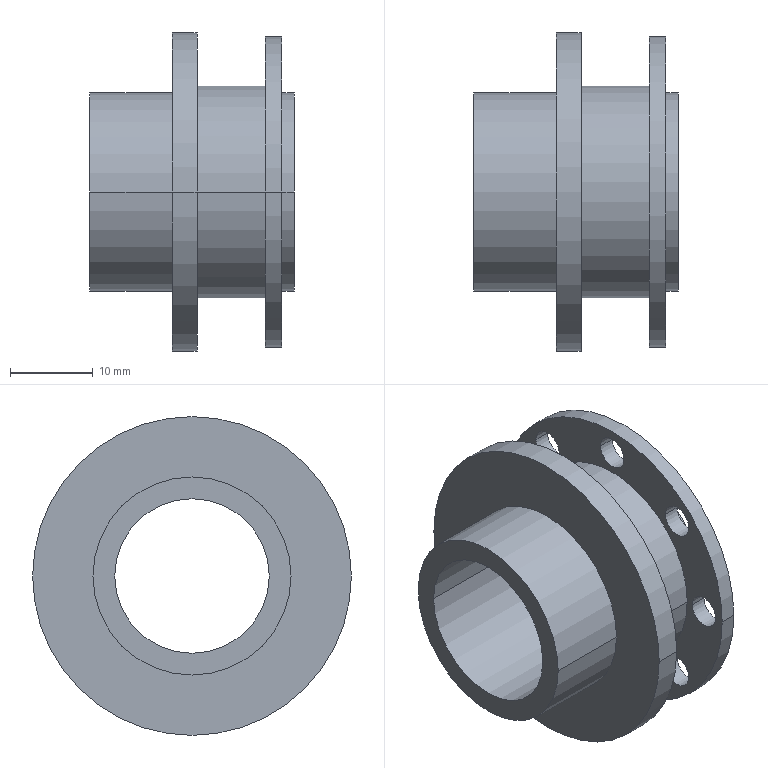Part | SolidWorks | features SavedExtBody 1 | 1 solid | 34 faces | box 24.772 x 38.609 x 38.609 mm | volume 8203 mm3 | cylinder 28 | plane 6 | commonest cylinder face diameters 4 x16 24 x4 18.724 x2 25.677 x2 37.649 x2 38.609 x2
STEP:
#1=CARTESIAN_POINT('',(-65.,13.695,65.));
#2=VERTEX_POINT('',#1);
#3=CARTESIAN_POINT('',(-65.,17.695,65.));
#4=VERTEX_POINT('',#3);
#5=CARTESIAN_POINT('',(-65.,15.695,65.));
#6=DIRECTION('',(1.,0.,0.));
#7=DIRECTION('',(0.,-1.,0.));
#8=AXIS2_PLACEMENT_3D('',#5,#6,#7);
#9=CIRCLE('',#8,2.);
#10=EDGE_CURVE('',#2,#4,#9,.T.);
#11=ORIENTED_EDGE('',*,*,#10,.T.);
#12=CARTESIAN_POINT('',(-67.,17.695,65.));
#13=VERTEX_POINT('',#12);
#14=CARTESIAN_POINT('',(-59.343,17.695,65.));
#15=DIRECTION('',(-1.,0.,0.));
#16=VECTOR('',#15,1000.);
#17=LINE('',#14,#16);
#18=EDGE_CURVE('',#4,#13,#17,.T.);
#19=ORIENTED_EDGE('',*,*,#18,.T.);
#20=CARTESIAN_POINT('',(-67.,13.695,65.));
#21=VERTEX_POINT('',#20);
#22=CARTESIAN_POINT('',(-67.,15.695,65.));
#23=DIRECTION('',(-1.,0.,0.));
#24=DIRECTION('',(0.,-1.,0.));
#25=AXIS2_PLACEMENT_3D('',#22,#23,#24);
#26=CIRCLE('',#25,2.);
#27=EDGE_CURVE('',#13,#21,#26,.T.);
#28=ORIENTED_EDGE('',*,*,#27,.T.);
#29=CARTESIAN_POINT('',(-59.343,13.695,65.));
#30=DIRECTION('',(-1.,0.,0.));
#31=VECTOR('',#30,1000.);
#32=LINE('',#29,#31);
#33=EDGE_CURVE('',#2,#21,#32,.T.);
#34=ORIENTED_EDGE('',*,*,#33,.F.);
#35=EDGE_LOOP('',(#11,#19,#28,#34));
#36=FACE_OUTER_BOUND('',#35,.T.);
#37=CARTESIAN_POINT('',(-59.343,15.695,65.));
#38=DIRECTION('',(-1.,0.,0.));
#39=DIRECTION('',(0.,-1.,0.));
#40=AXIS2_PLACEMENT_3D('',#37,#38,#39);
#41=CYLINDRICAL_SURFACE('',#40,2.);
#42=ADVANCED_FACE('',(#36),#41,.F.);
#43=CARTESIAN_POINT('',(-65.,9.098,76.098));
#44=VERTEX_POINT('',#43);
#45=CARTESIAN_POINT('',(-65.,13.098,76.098));
#46=VERTEX_POINT('',#45);
#47=CARTESIAN_POINT('',(-65.,11.098,76.098));
#48=DIRECTION('',(1.,0.,0.));
#49=DIRECTION('',(0.,-1.,0.));
#50=AXIS2_PLACEMENT_3D('',#47,#48,#49);
#51=CIRCLE('',#50,2.);
#52=EDGE_CURVE('',#44,#46,#51,.T.);
#53=ORIENTED_EDGE('',*,*,#52,.T.);
#54=CARTESIAN_POINT('',(-67.,13.098,76.098));
#55=VERTEX_POINT('',#54);
#56=CARTESIAN_POINT('',(-59.343,13.098,76.098));
#57=DIRECTION('',(-1.,0.,0.));
#58=VECTOR('',#57,1000.);
#59=LINE('',#56,#58);
#60=EDGE_CURVE('',#46,#55,#59,.T.);
#61=ORIENTED_EDGE('',*,*,#60,.T.);
#62=CARTESIAN_POINT('',(-67.,9.098,76.098));
#63=VERTEX_POINT('',#62);
#64=CARTESIAN_POINT('',(-67.,11.098,76.098));
#65=DIRECTION('',(-1.,0.,0.));
#66=DIRECTION('',(0.,-1.,0.));
#67=AXIS2_PLACEMENT_3D('',#64,#65,#66);
#68=CIRCLE('',#67,2.);
#69=EDGE_CURVE('',#55,#63,#68,.T.);
#70=ORIENTED_EDGE('',*,*,#69,.T.);
#71=CARTESIAN_POINT('',(-59.343,9.098,76.098));
#72=DIRECTION('',(-1.,0.,0.));
#73=VECTOR('',#72,1000.);
#74=LINE('',#71,#73);
#75=EDGE_CURVE('',#44,#63,#74,.T.);
#76=ORIENTED_EDGE('',*,*,#75,.F.);
#77=EDGE_LOOP('',(#53,#61,#70,#76));
#78=FACE_OUTER_BOUND('',#77,.T.);
#79=CARTESIAN_POINT('',(-59.343,11.098,76.098));
#80=DIRECTION('',(-1.,0.,0.));
#81=DIRECTION('',(0.,-1.,0.));
#82=AXIS2_PLACEMENT_3D('',#79,#80,#81);
#83=CYLINDRICAL_SURFACE('',#82,2.);
#84=ADVANCED_FACE('',(#78),#83,.F.);
#85=CARTESIAN_POINT('',(-65.,-2.,80.695));
#86=VERTEX_POINT('',#85);
#87=CARTESIAN_POINT('',(-65.,2.,80.695));
#88=VERTEX_POINT('',#87);
#89=CARTESIAN_POINT('',(-65.,0.,80.695));
#90=DIRECTION('',(1.,0.,0.));
#91=DIRECTION('',(0.,-1.,0.));
#92=AXIS2_PLACEMENT_3D('',#89,#90,#91);
#93=CIRCLE('',#92,2.);
#94=EDGE_CURVE('',#86,#88,#93,.T.);
#95=ORIENTED_EDGE('',*,*,#94,.T.);
#96=CARTESIAN_POINT('',(-67.,2.,80.695));
#97=VERTEX_POINT('',#96);
#98=CARTESIAN_POINT('',(-59.343,2.,80.695));
#99=DIRECTION('',(-1.,0.,0.));
#100=VECTOR('',#99,1000.);
#101=LINE('',#98,#100);
#102=EDGE_CURVE('',#88,#97,#101,.T.);
#103=ORIENTED_EDGE('',*,*,#102,.T.);
#104=CARTESIAN_POINT('',(-67.,-2.,80.695));
#105=VERTEX_POINT('',#104);
#106=CARTESIAN_POINT('',(-67.,0.,80.695));
#107=DIRECTION('',(-1.,0.,0.));
#108=DIRECTION('',(0.,-1.,0.));
#109=AXIS2_PLACEMENT_3D('',#106,#107,#108);
#110=CIRCLE('',#109,2.);
#111=EDGE_CURVE('',#97,#105,#110,.T.);
#112=ORIENTED_EDGE('',*,*,#111,.T.);
#113=CARTESIAN_POINT('',(-59.343,-2.,80.695));
#114=DIRECTION('',(-1.,0.,0.));
#115=VECTOR('',#114,1000.);
#116=LINE('',#113,#115);
#117=EDGE_CURVE('',#86,#105,#116,.T.);
#118=ORIENTED_EDGE('',*,*,#117,.F.);
#119=EDGE_LOOP('',(#95,#103,#112,#118));
#120=FACE_OUTER_BOUND('',#119,.T.);
#121=CARTESIAN_POINT('',(-59.343,0.,80.695));
#122=DIRECTION('',(-1.,0.,0.));
#123=DIRECTION('',(0.,-1.,0.));
#124=AXIS2_PLACEMENT_3D('',#121,#122,#123);
#125=CYLINDRICAL_SURFACE('',#124,2.);
#126=ADVANCED_FACE('',(#120),#125,.F.);
#127=CARTESIAN_POINT('',(-65.,-13.098,76.098));
#128=VERTEX_POINT('',#127);
#129=CARTESIAN_POINT('',(-65.,-9.098,76.098));
#130=VERTEX_POINT('',#129);
#131=CARTESIAN_POINT('',(-65.,-11.098,76.098));
#132=DIRECTION('',(1.,0.,0.));
#133=DIRECTION('',(0.,-1.,0.));
#134=AXIS2_PLACEMENT_3D('',#131,#132,#133);
#135=CIRCLE('',#134,2.);
#136=EDGE_CURVE('',#128,#130,#135,.T.);
#137=ORIENTED_EDGE('',*,*,#136,.T.);
#138=CARTESIAN_POINT('',(-67.,-9.098,76.098));
#139=VERTEX_POINT('',#138);
#140=CARTESIAN_POINT('',(-59.343,-9.098,76.098));
#141=DIRECTION('',(-1.,0.,0.));
#142=VECTOR('',#141,1000.);
#143=LINE('',#140,#142);
#144=EDGE_CURVE('',#130,#139,#143,.T.);
#145=ORIENTED_EDGE('',*,*,#144,.T.);
#146=CARTESIAN_POINT('',(-67.,-13.098,76.098));
#147=VERTEX_POINT('',#146);
#148=CARTESIAN_POINT('',(-67.,-11.098,76.098));
#149=DIRECTION('',(-1.,0.,0.));
#150=DIRECTION('',(0.,-1.,0.));
#151=AXIS2_PLACEMENT_3D('',#148,#149,#150);
#152=CIRCLE('',#151,2.);
#153=EDGE_CURVE('',#139,#147,#152,.T.);
#154=ORIENTED_EDGE('',*,*,#153,.T.);
#155=CARTESIAN_POINT('',(-59.343,-13.098,76.098));
#156=DIRECTION('',(-1.,0.,0.));
#157=VECTOR('',#156,1000.);
#158=LINE('',#155,#157);
#159=EDGE_CURVE('',#128,#147,#158,.T.);
#160=ORIENTED_EDGE('',*,*,#159,.F.);
#161=EDGE_LOOP('',(#137,#145,#154,#160));
#162=FACE_OUTER_BOUND('',#161,.T.);
#163=CARTESIAN_POINT('',(-59.343,-11.098,76.098));
#164=DIRECTION('',(-1.,0.,0.));
#165=DIRECTION('',(0.,-1.,0.));
#166=AXIS2_PLACEMENT_3D('',#163,#164,#165);
#167=CYLINDRICAL_SURFACE('',#166,2.);
#168=ADVANCED_FACE('',(#162),#167,.F.);
#169=CARTESIAN_POINT('',(-65.,-17.695,65.));
#170=VERTEX_POINT('',#169);
#171=CARTESIAN_POINT('',(-65.,-13.695,65.));
#172=VERTEX_POINT('',#171);
#173=CARTESIAN_POINT('',(-65.,-15.695,65.));
#174=DIRECTION('',(1.,0.,0.));
#175=DIRECTION('',(0.,-1.,0.));
#176=AXIS2_PLACEMENT_3D('',#173,#174,#175);
#177=CIRCLE('',#176,2.);
#178=EDGE_CURVE('',#170,#172,#177,.T.);
#179=ORIENTED_EDGE('',*,*,#178,.T.);
#180=CARTESIAN_POINT('',(-67.,-13.695,65.));
#181=VERTEX_POINT('',#180);
#182=CARTESIAN_POINT('',(-59.343,-13.695,65.));
#183=DIRECTION('',(-1.,0.,0.));
#184=VECTOR('',#183,1000.);
#185=LINE('',#182,#184);
#186=EDGE_CURVE('',#172,#181,#185,.T.);
#187=ORIENTED_EDGE('',*,*,#186,.T.);
#188=CARTESIAN_POINT('',(-67.,-17.695,65.));
#189=VERTEX_POINT('',#188);
#190=CARTESIAN_POINT('',(-67.,-15.695,65.));
#191=DIRECTION('',(-1.,0.,0.));
#192=DIRECTION('',(0.,-1.,0.));
#193=AXIS2_PLACEMENT_3D('',#190,#191,#192);
#194=CIRCLE('',#193,2.);
#195=EDGE_CURVE('',#181,#189,#194,.T.);
#196=ORIENTED_EDGE('',*,*,#195,.T.);
#197=CARTESIAN_POINT('',(-59.343,-17.695,65.));
#198=DIRECTION('',(-1.,0.,0.));
#199=VECTOR('',#198,1000.);
#200=LINE('',#197,#199);
#201=EDGE_CURVE('',#170,#189,#200,.T.);
#202=ORIENTED_EDGE('',*,*,#201,.F.);
#203=EDGE_LOOP('',(#179,#187,#196,#202));
#204=FACE_OUTER_BOUND('',#203,.T.);
#205=CARTESIAN_POINT('',(-59.343,-15.695,65.));
#206=DIRECTION('',(-1.,0.,0.));
#207=DIRECTION('',(0.,-1.,0.));
#208=AXIS2_PLACEMENT_3D('',#205,#206,#207);
#209=CYLINDRICAL_SURFACE('',#208,2.);
#210=ADVANCED_FACE('',(#204),#209,.F.);
#211=CARTESIAN_POINT('',(-65.,-13.098,53.902));
#212=VERTEX_POINT('',#211);
#213=CARTESIAN_POINT('',(-65.,-9.098,53.902));
#214=VERTEX_POINT('',#213);
#215=CARTESIAN_POINT('',(-65.,-11.098,53.902));
#216=DIRECTION('',(1.,0.,0.));
#217=DIRECTION('',(0.,-1.,0.));
#218=AXIS2_PLACEMENT_3D('',#215,#216,#217);
#219=CIRCLE('',#218,2.);
#220=EDGE_CURVE('',#212,#214,#219,.T.);
#221=ORIENTED_EDGE('',*,*,#220,.T.);
#222=CARTESIAN_POINT('',(-67.,-9.098,53.902));
#223=VERTEX_POINT('',#222);
#224=CARTESIAN_POINT('',(-59.343,-9.098,53.902));
#225=DIRECTION('',(-1.,0.,0.));
#226=VECTOR('',#225,1000.);
#227=LINE('',#224,#226);
#228=EDGE_CURVE('',#214,#223,#227,.T.);
#229=ORIENTED_EDGE('',*,*,#228,.T.);
#230=CARTESIAN_POINT('',(-67.,-13.098,53.902));
#231=VERTEX_POINT('',#230);
#232=CARTESIAN_POINT('',(-67.,-11.098,53.902));
#233=DIRECTION('',(-1.,0.,0.));
#234=DIRECTION('',(0.,-1.,0.));
#235=AXIS2_PLACEMENT_3D('',#232,#233,#234);
#236=CIRCLE('',#235,2.);
#237=EDGE_CURVE('',#223,#231,#236,.T.);
#238=ORIENTED_EDGE('',*,*,#237,.T.);
#239=CARTESIAN_POINT('',(-59.343,-13.098,53.902));
#240=DIRECTION('',(-1.,0.,0.));
#241=VECTOR('',#240,1000.);
#242=LINE('',#239,#241);
#243=EDGE_CURVE('',#212,#231,#242,.T.);
#244=ORIENTED_EDGE('',*,*,#243,.F.);
#245=EDGE_LOOP('',(#221,#229,#238,#244));
#246=FACE_OUTER_BOUND('',#245,.T.);
#247=CARTESIAN_POINT('',(-59.343,-11.098,53.902));
#248=DIRECTION('',(-1.,0.,0.));
#249=DIRECTION('',(0.,-1.,0.));
#250=AXIS2_PLACEMENT_3D('',#247,#248,#249);
#251=CYLINDRICAL_SURFACE('',#250,2.);
#252=ADVANCED_FACE('',(#246),#251,.F.);
#253=CARTESIAN_POINT('',(-65.,-2.,49.305));
#254=VERTEX_POINT('',#253);
#255=CARTESIAN_POINT('',(-65.,2.,49.305));
#256=VERTEX_POINT('',#255);
#257=CARTESIAN_POINT('',(-65.,0.,49.305));
#258=DIRECTION('',(1.,0.,0.));
#259=DIRECTION('',(0.,-1.,0.));
#260=AXIS2_PLACEMENT_3D('',#257,#258,#259);
#261=CIRCLE('',#260,2.);
#262=EDGE_CURVE('',#254,#256,#261,.T.);
#263=ORIENTED_EDGE('',*,*,#262,.T.);
#264=CARTESIAN_POINT('',(-67.,2.,49.305));
#265=VERTEX_POINT('',#264);
#266=CARTESIAN_POINT('',(-59.343,2.,49.305));
#267=DIRECTION('',(-1.,0.,0.));
#268=VECTOR('',#267,1000.);
#269=LINE('',#266,#268);
#270=EDGE_CURVE('',#256,#265,#269,.T.);
#271=ORIENTED_EDGE('',*,*,#270,.T.);
#272=CARTESIAN_POINT('',(-67.,-2.,49.305));
#273=VERTEX_POINT('',#272);
#274=CARTESIAN_POINT('',(-67.,0.,49.305));
#275=DIRECTION('',(-1.,0.,0.));
#276=DIRECTION('',(0.,-1.,0.));
#277=AXIS2_PLACEMENT_3D('',#274,#275,#276);
#278=CIRCLE('',#277,2.);
#279=EDGE_CURVE('',#265,#273,#278,.T.);
#280=ORIENTED_EDGE('',*,*,#279,.T.);
#281=CARTESIAN_POINT('',(-59.343,-2.,49.305));
#282=DIRECTION('',(-1.,0.,0.));
#283=VECTOR('',#282,1000.);
#284=LINE('',#281,#283);
#285=EDGE_CURVE('',#254,#273,#284,.T.);
#286=ORIENTED_EDGE('',*,*,#285,.F.);
#287=EDGE_LOOP('',(#263,#271,#280,#286));
#288=FACE_OUTER_BOUND('',#287,.T.);
#289=CARTESIAN_POINT('',(-59.343,0.,49.305));
#290=DIRECTION('',(-1.,0.,0.));
#291=DIRECTION('',(0.,-1.,0.));
#292=AXIS2_PLACEMENT_3D('',#289,#290,#291);
#293=CYLINDRICAL_SURFACE('',#292,2.);
#294=ADVANCED_FACE('',(#288),#293,.F.);
#295=CARTESIAN_POINT('',(-65.,9.098,53.902));
#296=VERTEX_POINT('',#295);
#297=CARTESIAN_POINT('',(-65.,13.098,53.902));
#298=VERTEX_POINT('',#297);
#299=CARTESIAN_POINT('',(-65.,11.098,53.902));
#300=DIRECTION('',(1.,0.,0.));
#301=DIRECTION('',(0.,-1.,0.));
#302=AXIS2_PLACEMENT_3D('',#299,#300,#301);
#303=CIRCLE('',#302,2.);
#304=EDGE_CURVE('',#296,#298,#303,.T.);
#305=ORIENTED_EDGE('',*,*,#304,.T.);
#306=CARTESIAN_POINT('',(-67.,13.098,53.902));
#307=VERTEX_POINT('',#306);
#308=CARTESIAN_POINT('',(-59.343,13.098,53.902));
#309=DIRECTION('',(-1.,0.,0.));
#310=VECTOR('',#309,1000.);
#311=LINE('',#308,#310);
#312=EDGE_CURVE('',#298,#307,#311,.T.);
#313=ORIENTED_EDGE('',*,*,#312,.T.);
#314=CARTESIAN_POINT('',(-67.,9.098,53.902));
#315=VERTEX_POINT('',#314);
#316=CARTESIAN_POINT('',(-67.,11.098,53.902));
#317=DIRECTION('',(-1.,0.,0.));
#318=DIRECTION('',(0.,-1.,0.));
#319=AXIS2_PLACEMENT_3D('',#316,#317,#318);
#320=CIRCLE('',#319,2.);
#321=EDGE_CURVE('',#307,#315,#320,.T.);
#322=ORIENTED_EDGE('',*,*,#321,.T.);
#323=CARTESIAN_POINT('',(-59.343,9.098,53.902));
#324=DIRECTION('',(-1.,0.,0.));
#325=VECTOR('',#324,1000.);
#326=LINE('',#323,#325);
#327=EDGE_CURVE('',#296,#315,#326,.T.);
#328=ORIENTED_EDGE('',*,*,#327,.F.);
#329=EDGE_LOOP('',(#305,#313,#322,#328));
#330=FACE_OUTER_BOUND('',#329,.T.);
#331=CARTESIAN_POINT('',(-59.343,11.098,53.902));
#332=DIRECTION('',(-1.,0.,0.));
#333=DIRECTION('',(0.,-1.,0.));
#334=AXIS2_PLACEMENT_3D('',#331,#332,#333);
#335=CYLINDRICAL_SURFACE('',#334,2.);
#336=ADVANCED_FACE('',(#330),#335,.F.);
#337=CARTESIAN_POINT('',(-78.272,-12.,65.));
#338=VERTEX_POINT('',#337);
#339=CARTESIAN_POINT('',(-78.272,12.,65.));
#340=VERTEX_POINT('',#339);
#341=CARTESIAN_POINT('',(-78.272,0.,65.));
#342=DIRECTION('',(-1.,0.,0.));
#343=DIRECTION('',(0.,-1.,0.));
#344=AXIS2_PLACEMENT_3D('',#341,#342,#343);
#345=CIRCLE('',#344,12.);
#346=EDGE_CURVE('',#338,#340,#345,.T.);
#347=ORIENTED_EDGE('',*,*,#346,.T.);
#348=CARTESIAN_POINT('',(-88.272,12.,65.));
#349=VERTEX_POINT('',#348);
#350=CARTESIAN_POINT('',(-88.272,12.,65.));
#351=DIRECTION('',(-1.,0.,0.));
#352=VECTOR('',#351,1000.);
#353=LINE('',#350,#352);
#354=EDGE_CURVE('',#340,#349,#353,.T.);
#355=ORIENTED_EDGE('',*,*,#354,.T.);
#356=CARTESIAN_POINT('',(-88.272,-12.,65.));
#357=VERTEX_POINT('',#356);
#358=CARTESIAN_POINT('',(-88.272,0.,65.));
#359=DIRECTION('',(-1.,0.,0.));
#360=DIRECTION('',(0.,-1.,0.));
#361=AXIS2_PLACEMENT_3D('',#358,#359,#360);
#362=CIRCLE('',#361,12.);
#363=EDGE_CURVE('',#357,#349,#362,.T.);
#364=ORIENTED_EDGE('',*,*,#363,.F.);
#365=CARTESIAN_POINT('',(-88.272,-12.,65.));
#366=DIRECTION('',(-1.,0.,0.));
#367=VECTOR('',#366,1000.);
#368=LINE('',#365,#367);
#369=EDGE_CURVE('',#338,#357,#368,.T.);
#370=ORIENTED_EDGE('',*,*,#369,.F.);
#371=EDGE_LOOP('',(#347,#355,#364,#370));
#372=FACE_OUTER_BOUND('',#371,.T.);
#373=CARTESIAN_POINT('',(-88.272,0.,65.));
#374=DIRECTION('',(-1.,0.,0.));
#375=DIRECTION('',(0.,-1.,0.));
#376=AXIS2_PLACEMENT_3D('',#373,#374,#375);
#377=CYLINDRICAL_SURFACE('',#376,12.);
#378=ADVANCED_FACE('',(#372),#377,.T.);
#379=CARTESIAN_POINT('',(-75.272,-19.305,65.));
#380=VERTEX_POINT('',#379);
#381=CARTESIAN_POINT('',(-75.272,19.305,65.));
#382=VERTEX_POINT('',#381);
#383=CARTESIAN_POINT('',(-75.272,0.,65.));
#384=DIRECTION('',(-1.,0.,0.));
#385=DIRECTION('',(0.,-1.,0.));
#386=AXIS2_PLACEMENT_3D('',#383,#384,#385);
#387=CIRCLE('',#386,19.305);
#388=EDGE_CURVE('',#380,#382,#387,.T.);
#389=ORIENTED_EDGE('',*,*,#388,.T.);
#390=CARTESIAN_POINT('',(-78.272,19.305,65.));
#391=VERTEX_POINT('',#390);
#392=CARTESIAN_POINT('',(-88.272,19.305,65.));
#393=DIRECTION('',(-1.,0.,0.));
#394=VECTOR('',#393,1000.);
#395=LINE('',#392,#394);
#396=EDGE_CURVE('',#382,#391,#395,.T.);
#397=ORIENTED_EDGE('',*,*,#396,.T.);
#398=CARTESIAN_POINT('',(-78.272,-19.305,65.));
#399=VERTEX_POINT('',#398);
#400=CARTESIAN_POINT('',(-78.272,0.,65.));
#401=DIRECTION('',(-1.,0.,0.));
#402=DIRECTION('',(0.,-1.,0.));
#403=AXIS2_PLACEMENT_3D('',#400,#401,#402);
#404=CIRCLE('',#403,19.305);
#405=EDGE_CURVE('',#399,#391,#404,.T.);
#406=ORIENTED_EDGE('',*,*,#405,.F.);
#407=CARTESIAN_POINT('',(-88.272,-19.305,65.));
#408=DIRECTION('',(-1.,0.,0.));
#409=VECTOR('',#408,1000.);
#410=LINE('',#407,#409);
#411=EDGE_CURVE('',#380,#399,#410,.T.);
#412=ORIENTED_EDGE('',*,*,#411,.F.);
#413=EDGE_LOOP('',(#389,#397,#406,#412));
#414=FACE_OUTER_BOUND('',#413,.T.);
#415=CARTESIAN_POINT('',(-88.272,0.,65.));
#416=DIRECTION('',(-1.,0.,0.));
#417=DIRECTION('',(0.,-1.,0.));
#418=AXIS2_PLACEMENT_3D('',#415,#416,#417);
#419=CYLINDRICAL_SURFACE('',#418,19.305);
#420=ADVANCED_FACE('',(#414),#419,.T.);
#421=CARTESIAN_POINT('',(-67.,-12.839,65.));
#422=VERTEX_POINT('',#421);
#423=CARTESIAN_POINT('',(-67.,12.839,65.));
#424=VERTEX_POINT('',#423);
#425=CARTESIAN_POINT('',(-67.,0.,65.));
#426=DIRECTION('',(-1.,0.,0.));
#427=DIRECTION('',(0.,-1.,0.));
#428=AXIS2_PLACEMENT_3D('',#425,#426,#427);
#429=CIRCLE('',#428,12.839);
#430=EDGE_CURVE('',#422,#424,#429,.T.);
#431=ORIENTED_EDGE('',*,*,#430,.T.);
#432=CARTESIAN_POINT('',(-75.272,12.839,65.));
#433=VERTEX_POINT('',#432);
#434=CARTESIAN_POINT('',(-88.272,12.839,65.));
#435=DIRECTION('',(-1.,0.,0.));
#436=VECTOR('',#435,1000.);
#437=LINE('',#434,#436);
#438=EDGE_CURVE('',#424,#433,#437,.T.);
#439=ORIENTED_EDGE('',*,*,#438,.T.);
#440=CARTESIAN_POINT('',(-75.272,-12.839,65.));
#441=VERTEX_POINT('',#440);
#442=CARTESIAN_POINT('',(-75.272,0.,65.));
#443=DIRECTION('',(-1.,0.,0.));
#444=DIRECTION('',(0.,-1.,0.));
#445=AXIS2_PLACEMENT_3D('',#442,#443,#444);
#446=CIRCLE('',#445,12.839);
#447=EDGE_CURVE('',#441,#433,#446,.T.);
#448=ORIENTED_EDGE('',*,*,#447,.F.);
#449=CARTESIAN_POINT('',(-88.272,-12.839,65.));
#450=DIRECTION('',(-1.,0.,0.));
#451=VECTOR('',#450,1000.);
#452=LINE('',#449,#451);
#453=EDGE_CURVE('',#422,#441,#452,.T.);
#454=ORIENTED_EDGE('',*,*,#453,.F.);
#455=EDGE_LOOP('',(#431,#439,#448,#454));
#456=FACE_OUTER_BOUND('',#455,.T.);
#457=CARTESIAN_POINT('',(-88.272,0.,65.));
#458=DIRECTION('',(-1.,0.,0.));
#459=DIRECTION('',(0.,-1.,0.));
#460=AXIS2_PLACEMENT_3D('',#457,#458,#459);
#461=CYLINDRICAL_SURFACE('',#460,12.839);
#462=ADVANCED_FACE('',(#456),#461,.T.);
#463=CARTESIAN_POINT('',(-65.,-18.825,65.));
#464=VERTEX_POINT('',#463);
#465=CARTESIAN_POINT('',(-65.,18.825,65.));
#466=VERTEX_POINT('',#465);
#467=CARTESIAN_POINT('',(-65.,0.,65.));
#468=DIRECTION('',(-1.,0.,0.));
#469=DIRECTION('',(0.,-1.,0.));
#470=AXIS2_PLACEMENT_3D('',#467,#468,#469);
#471=CIRCLE('',#470,18.825);
#472=EDGE_CURVE('',#464,#466,#471,.T.);
#473=ORIENTED_EDGE('',*,*,#472,.T.);
#474=CARTESIAN_POINT('',(-67.,18.825,65.));
#475=VERTEX_POINT('',#474);
#476=CARTESIAN_POINT('',(-88.272,18.825,65.));
#477=DIRECTION('',(-1.,0.,0.));
#478=VECTOR('',#477,1000.);
#479=LINE('',#476,#478);
#480=EDGE_CURVE('',#466,#475,#479,.T.);
#481=ORIENTED_EDGE('',*,*,#480,.T.);
#482=CARTESIAN_POINT('',(-67.,-18.825,65.));
#483=VERTEX_POINT('',#482);
#484=CARTESIAN_POINT('',(-67.,0.,65.));
#485=DIRECTION('',(-1.,0.,0.));
#486=DIRECTION('',(0.,-1.,0.));
#487=AXIS2_PLACEMENT_3D('',#484,#485,#486);
#488=CIRCLE('',#487,18.825);
#489=EDGE_CURVE('',#483,#475,#488,.T.);
#490=ORIENTED_EDGE('',*,*,#489,.F.);
#491=CARTESIAN_POINT('',(-88.272,-18.825,65.));
#492=DIRECTION('',(-1.,0.,0.));
#493=VECTOR('',#492,1000.);
#494=LINE('',#491,#493);
#495=EDGE_CURVE('',#464,#483,#494,.T.);
#496=ORIENTED_EDGE('',*,*,#495,.F.);
#497=EDGE_LOOP('',(#473,#481,#490,#496));
#498=FACE_OUTER_BOUND('',#497,.T.);
#499=CARTESIAN_POINT('',(-88.272,0.,65.));
#500=DIRECTION('',(-1.,0.,0.));
#501=DIRECTION('',(0.,-1.,0.));
#502=AXIS2_PLACEMENT_3D('',#499,#500,#501);
#503=CYLINDRICAL_SURFACE('',#502,18.825);
#504=ADVANCED_FACE('',(#498),#503,.T.);
#505=CARTESIAN_POINT('',(-63.5,-12.,65.));
#506=VERTEX_POINT('',#505);
#507=CARTESIAN_POINT('',(-63.5,12.,65.));
#508=VERTEX_POINT('',#507);
#509=CARTESIAN_POINT('',(-63.5,0.,65.));
#510=DIRECTION('',(-1.,0.,0.));
#511=DIRECTION('',(0.,-1.,0.));
#512=AXIS2_PLACEMENT_3D('',#509,#510,#511);
#513=CIRCLE('',#512,12.);
#514=EDGE_CURVE('',#506,#508,#513,.T.);
#515=ORIENTED_EDGE('',*,*,#514,.T.);
#516=CARTESIAN_POINT('',(-65.,12.,65.));
#517=VERTEX_POINT('',#516);
#518=CARTESIAN_POINT('',(-88.272,12.,65.));
#519=DIRECTION('',(-1.,0.,0.));
#520=VECTOR('',#519,1000.);
#521=LINE('',#518,#520);
#522=EDGE_CURVE('',#508,#517,#521,.T.);
#523=ORIENTED_EDGE('',*,*,#522,.T.);
#524=CARTESIAN_POINT('',(-65.,-12.,65.));
#525=VERTEX_POINT('',#524);
#526=CARTESIAN_POINT('',(-65.,0.,65.));
#527=DIRECTION('',(-1.,0.,0.));
#528=DIRECTION('',(0.,-1.,0.));
#529=AXIS2_PLACEMENT_3D('',#526,#527,#528);
#530=CIRCLE('',#529,12.);
#531=EDGE_CURVE('',#525,#517,#530,.T.);
#532=ORIENTED_EDGE('',*,*,#531,.F.);
#533=CARTESIAN_POINT('',(-88.272,-12.,65.));
#534=DIRECTION('',(-1.,0.,0.));
#535=VECTOR('',#534,1000.);
#536=LINE('',#533,#535);
#537=EDGE_CURVE('',#506,#525,#536,.T.);
#538=ORIENTED_EDGE('',*,*,#537,.F.);
#539=EDGE_LOOP('',(#515,#523,#532,#538));
#540=FACE_OUTER_BOUND('',#539,.T.);
#541=CARTESIAN_POINT('',(-88.272,0.,65.));
#542=DIRECTION('',(-1.,0.,0.));
#543=DIRECTION('',(0.,-1.,0.));
#544=AXIS2_PLACEMENT_3D('',#541,#542,#543);
#545=CYLINDRICAL_SURFACE('',#544,12.);
#546=ADVANCED_FACE('',(#540),#545,.T.);
#547=CARTESIAN_POINT('',(-63.5,9.362,65.));
#548=VERTEX_POINT('',#547);
#549=CARTESIAN_POINT('',(-63.5,-9.362,65.));
#550=VERTEX_POINT('',#549);
#551=CARTESIAN_POINT('',(-63.5,0.,65.));
#552=DIRECTION('',(-1.,0.,0.));
#553=DIRECTION('',(0.,-1.,0.));
#554=AXIS2_PLACEMENT_3D('',#551,#552,#553);
#555=CIRCLE('',#554,9.362);
#556=EDGE_CURVE('',#548,#550,#555,.T.);
#557=ORIENTED_EDGE('',*,*,#556,.F.);
#558=CARTESIAN_POINT('',(-88.272,9.362,65.));
#559=VERTEX_POINT('',#558);
#560=CARTESIAN_POINT('',(-88.272,9.362,65.));
#561=DIRECTION('',(-1.,0.,0.));
#562=VECTOR('',#561,1000.);
#563=LINE('',#560,#562);
#564=EDGE_CURVE('',#548,#559,#563,.T.);
#565=ORIENTED_EDGE('',*,*,#564,.T.);
#566=CARTESIAN_POINT('',(-88.272,-9.362,65.));
#567=VERTEX_POINT('',#566);
#568=CARTESIAN_POINT('',(-88.272,0.,65.));
#569=DIRECTION('',(-1.,0.,0.));
#570=DIRECTION('',(0.,-1.,0.));
#571=AXIS2_PLACEMENT_3D('',#568,#569,#570);
#572=CIRCLE('',#571,9.362);
#573=EDGE_CURVE('',#559,#567,#572,.T.);
#574=ORIENTED_EDGE('',*,*,#573,.T.);
#575=CARTESIAN_POINT('',(-88.272,-9.362,65.));
#576=DIRECTION('',(-1.,0.,0.));
#577=VECTOR('',#576,1000.);
#578=LINE('',#575,#577);
#579=EDGE_CURVE('',#550,#567,#578,.T.);
#580=ORIENTED_EDGE('',*,*,#579,.F.);
#581=EDGE_LOOP('',(#557,#565,#574,#580));
#582=FACE_OUTER_BOUND('',#581,.T.);
#583=CARTESIAN_POINT('',(-88.272,0.,65.));
#584=DIRECTION('',(-1.,0.,0.));
#585=DIRECTION('',(0.,-1.,0.));
#586=AXIS2_PLACEMENT_3D('',#583,#584,#585);
#587=CYLINDRICAL_SURFACE('',#586,9.362);
#588=ADVANCED_FACE('',(#582),#587,.F.);
#589=ORIENTED_EDGE('',*,*,#564,.F.);
#590=CARTESIAN_POINT('',(-63.5,0.,65.));
#591=DIRECTION('',(-1.,0.,0.));
#592=DIRECTION('',(0.,-1.,0.));
#593=AXIS2_PLACEMENT_3D('',#590,#591,#592);
#594=CIRCLE('',#593,9.362);
#595=EDGE_CURVE('',#550,#548,#594,.T.);
#596=ORIENTED_EDGE('',*,*,#595,.F.);
#597=ORIENTED_EDGE('',*,*,#579,.T.);
#598=CARTESIAN_POINT('',(-88.272,0.,65.));
#599=DIRECTION('',(-1.,0.,0.));
#600=DIRECTION('',(0.,-1.,0.));
#601=AXIS2_PLACEMENT_3D('',#598,#599,#600);
#602=CIRCLE('',#601,9.362);
#603=EDGE_CURVE('',#567,#559,#602,.T.);
#604=ORIENTED_EDGE('',*,*,#603,.T.);
#605=EDGE_LOOP('',(#589,#596,#597,#604));
#606=FACE_OUTER_BOUND('',#605,.T.);
#607=CARTESIAN_POINT('',(-88.272,0.,65.));
#608=DIRECTION('',(-1.,0.,0.));
#609=DIRECTION('',(0.,-1.,0.));
#610=AXIS2_PLACEMENT_3D('',#607,#608,#609);
#611=CYLINDRICAL_SURFACE('',#610,9.362);
#612=ADVANCED_FACE('',(#606),#611,.F.);
#613=ORIENTED_EDGE('',*,*,#595,.T.);
#614=ORIENTED_EDGE('',*,*,#556,.T.);
#615=EDGE_LOOP('',(#613,#614));
#616=FACE_BOUND('',#615,.T.);
#617=ORIENTED_EDGE('',*,*,#514,.F.);
#618=CARTESIAN_POINT('',(-63.5,0.,65.));
#619=DIRECTION('',(-1.,0.,0.));
#620=DIRECTION('',(0.,-1.,0.));
#621=AXIS2_PLACEMENT_3D('',#618,#619,#620);
#622=CIRCLE('',#621,12.);
#623=EDGE_CURVE('',#508,#506,#622,.T.);
#624=ORIENTED_EDGE('',*,*,#623,.F.);
#625=EDGE_LOOP('',(#617,#624));
#626=FACE_OUTER_BOUND('',#625,.T.);
#627=CARTESIAN_POINT('',(-63.5,0.,65.));
#628=DIRECTION('',(1.,0.,0.));
#629=DIRECTION('',(0.,1.,0.));
#630=AXIS2_PLACEMENT_3D('',#627,#628,#629);
#631=PLANE('',#630);
#632=ADVANCED_FACE('',(#616,#626),#631,.T.);
#633=ORIENTED_EDGE('',*,*,#522,.F.);
#634=ORIENTED_EDGE('',*,*,#623,.T.);
#635=ORIENTED_EDGE('',*,*,#537,.T.);
#636=CARTESIAN_POINT('',(-65.,0.,65.));
#637=DIRECTION('',(-1.,0.,0.));
#638=DIRECTION('',(0.,-1.,0.));
#639=AXIS2_PLACEMENT_3D('',#636,#637,#638);
#640=CIRCLE('',#639,12.);
#641=EDGE_CURVE('',#517,#525,#640,.T.);
#642=ORIENTED_EDGE('',*,*,#641,.F.);
#643=EDGE_LOOP('',(#633,#634,#635,#642));
#644=FACE_OUTER_BOUND('',#643,.T.);
#645=CARTESIAN_POINT('',(-88.272,0.,65.));
#646=DIRECTION('',(-1.,0.,0.));
#647=DIRECTION('',(0.,-1.,0.));
#648=AXIS2_PLACEMENT_3D('',#645,#646,#647);
#649=CYLINDRICAL_SURFACE('',#648,12.);
#650=ADVANCED_FACE('',(#644),#649,.T.);
#651=ORIENTED_EDGE('',*,*,#10,.F.);
#652=CARTESIAN_POINT('',(-65.,15.695,65.));
#653=DIRECTION('',(1.,0.,0.));
#654=DIRECTION('',(0.,-1.,0.));
#655=AXIS2_PLACEMENT_3D('',#652,#653,#654);
#656=CIRCLE('',#655,2.);
#657=EDGE_CURVE('',#4,#2,#656,.T.);
#658=ORIENTED_EDGE('',*,*,#657,.F.);
#659=EDGE_LOOP('',(#651,#658));
#660=FACE_BOUND('',#659,.T.);
#661=ORIENTED_EDGE('',*,*,#52,.F.);
#662=CARTESIAN_POINT('',(-65.,11.098,76.098));
#663=DIRECTION('',(1.,0.,0.));
#664=DIRECTION('',(0.,-1.,0.));
#665=AXIS2_PLACEMENT_3D('',#662,#663,#664);
#666=CIRCLE('',#665,2.);
#667=EDGE_CURVE('',#46,#44,#666,.T.);
#668=ORIENTED_EDGE('',*,*,#667,.F.);
#669=EDGE_LOOP('',(#661,#668));
#670=FACE_BOUND('',#669,.T.);
#671=ORIENTED_EDGE('',*,*,#94,.F.);
#672=CARTESIAN_POINT('',(-65.,0.,80.695));
#673=DIRECTION('',(1.,0.,0.));
#674=DIRECTION('',(0.,-1.,0.));
#675=AXIS2_PLACEMENT_3D('',#672,#673,#674);
#676=CIRCLE('',#675,2.);
#677=EDGE_CURVE('',#88,#86,#676,.T.);
#678=ORIENTED_EDGE('',*,*,#677,.F.);
#679=EDGE_LOOP('',(#671,#678));
#680=FACE_BOUND('',#679,.T.);
#681=ORIENTED_EDGE('',*,*,#136,.F.);
#682=CARTESIAN_POINT('',(-65.,-11.098,76.098));
#683=DIRECTION('',(1.,0.,0.));
#684=DIRECTION('',(0.,-1.,0.));
#685=AXIS2_PLACEMENT_3D('',#682,#683,#684);
#686=CIRCLE('',#685,2.);
#687=EDGE_CURVE('',#130,#128,#686,.T.);
#688=ORIENTED_EDGE('',*,*,#687,.F.);
#689=EDGE_LOOP('',(#681,#688));
#690=FACE_BOUND('',#689,.T.);
#691=ORIENTED_EDGE('',*,*,#178,.F.);
#692=CARTESIAN_POINT('',(-65.,-15.695,65.));
#693=DIRECTION('',(1.,0.,0.));
#694=DIRECTION('',(0.,-1.,0.));
#695=AXIS2_PLACEMENT_3D('',#692,#693,#694);
#696=CIRCLE('',#695,2.);
#697=EDGE_CURVE('',#172,#170,#696,.T.);
#698=ORIENTED_EDGE('',*,*,#697,.F.);
#699=EDGE_LOOP('',(#691,#698));
#700=FACE_BOUND('',#699,.T.);
#701=ORIENTED_EDGE('',*,*,#220,.F.);
#702=CARTESIAN_POINT('',(-65.,-11.098,53.902));
#703=DIRECTION('',(1.,0.,0.));
#704=DIRECTION('',(0.,-1.,0.));
#705=AXIS2_PLACEMENT_3D('',#702,#703,#704);
#706=CIRCLE('',#705,2.);
#707=EDGE_CURVE('',#214,#212,#706,.T.);
#708=ORIENTED_EDGE('',*,*,#707,.F.);
#709=EDGE_LOOP('',(#701,#708));
#710=FACE_BOUND('',#709,.T.);
#711=ORIENTED_EDGE('',*,*,#262,.F.);
#712=CARTESIAN_POINT('',(-65.,0.,49.305));
#713=DIRECTION('',(1.,0.,0.));
#714=DIRECTION('',(0.,-1.,0.));
#715=AXIS2_PLACEMENT_3D('',#712,#713,#714);
#716=CIRCLE('',#715,2.);
#717=EDGE_CURVE('',#256,#254,#716,.T.);
#718=ORIENTED_EDGE('',*,*,#717,.F.);
#719=EDGE_LOOP('',(#711,#718));
#720=FACE_BOUND('',#719,.T.);
#721=ORIENTED_EDGE('',*,*,#304,.F.);
#722=CARTESIAN_POINT('',(-65.,11.098,53.902));
#723=DIRECTION('',(1.,0.,0.));
#724=DIRECTION('',(0.,-1.,0.));
#725=AXIS2_PLACEMENT_3D('',#722,#723,#724);
#726=CIRCLE('',#725,2.);
#727=EDGE_CURVE('',#298,#296,#726,.T.);
#728=ORIENTED_EDGE('',*,*,#727,.F.);
#729=EDGE_LOOP('',(#721,#728));
#730=FACE_BOUND('',#729,.T.);
#731=ORIENTED_EDGE('',*,*,#472,.F.);
#732=CARTESIAN_POINT('',(-65.,0.,65.));
#733=DIRECTION('',(-1.,0.,0.));
#734=DIRECTION('',(0.,-1.,0.));
#735=AXIS2_PLACEMENT_3D('',#732,#733,#734);
#736=CIRCLE('',#735,18.825);
#737=EDGE_CURVE('',#466,#464,#736,.T.);
#738=ORIENTED_EDGE('',*,*,#737,.F.);
#739=EDGE_LOOP('',(#731,#738));
#740=FACE_OUTER_BOUND('',#739,.T.);
#741=ORIENTED_EDGE('',*,*,#531,.T.);
#742=ORIENTED_EDGE('',*,*,#641,.T.);
#743=EDGE_LOOP('',(#741,#742));
#744=FACE_BOUND('',#743,.T.);
#745=CARTESIAN_POINT('',(-65.,0.,65.));
#746=DIRECTION('',(-1.,0.,0.));
#747=DIRECTION('',(0.,-1.,0.));
#748=AXIS2_PLACEMENT_3D('',#745,#746,#747);
#749=PLANE('',#748);
#750=ADVANCED_FACE('',(#660,#670,#680,#690,#700,#710,#720,#730,#740,#744),#749,.F.);
#751=ORIENTED_EDGE('',*,*,#480,.F.);
#752=ORIENTED_EDGE('',*,*,#737,.T.);
#753=ORIENTED_EDGE('',*,*,#495,.T.);
#754=CARTESIAN_POINT('',(-67.,0.,65.));
#755=DIRECTION('',(-1.,0.,0.));
#756=DIRECTION('',(0.,-1.,0.));
#757=AXIS2_PLACEMENT_3D('',#754,#755,#756);
#758=CIRCLE('',#757,18.825);
#759=EDGE_CURVE('',#475,#483,#758,.T.);
#760=ORIENTED_EDGE('',*,*,#759,.F.);
#761=EDGE_LOOP('',(#751,#752,#753,#760));
#762=FACE_OUTER_BOUND('',#761,.T.);
#763=CARTESIAN_POINT('',(-88.272,0.,65.));
#764=DIRECTION('',(-1.,0.,0.));
#765=DIRECTION('',(0.,-1.,0.));
#766=AXIS2_PLACEMENT_3D('',#763,#764,#765);
#767=CYLINDRICAL_SURFACE('',#766,18.825);
#768=ADVANCED_FACE('',(#762),#767,.T.);
#769=CARTESIAN_POINT('',(-67.,15.695,65.));
#770=DIRECTION('',(-1.,0.,0.));
#771=DIRECTION('',(0.,-1.,0.));
#772=AXIS2_PLACEMENT_3D('',#769,#770,#771);
#773=CIRCLE('',#772,2.);
#774=EDGE_CURVE('',#21,#13,#773,.T.);
#775=ORIENTED_EDGE('',*,*,#774,.F.);
#776=ORIENTED_EDGE('',*,*,#27,.F.);
#777=EDGE_LOOP('',(#775,#776));
#778=FACE_BOUND('',#777,.T.);
#779=CARTESIAN_POINT('',(-67.,11.098,76.098));
#780=DIRECTION('',(-1.,0.,0.));
#781=DIRECTION('',(0.,-1.,0.));
#782=AXIS2_PLACEMENT_3D('',#779,#780,#781);
#783=CIRCLE('',#782,2.);
#784=EDGE_CURVE('',#63,#55,#783,.T.);
#785=ORIENTED_EDGE('',*,*,#784,.F.);
#786=ORIENTED_EDGE('',*,*,#69,.F.);
#787=EDGE_LOOP('',(#785,#786));
#788=FACE_BOUND('',#787,.T.);
#789=CARTESIAN_POINT('',(-67.,0.,80.695));
#790=DIRECTION('',(-1.,0.,0.));
#791=DIRECTION('',(0.,-1.,0.));
#792=AXIS2_PLACEMENT_3D('',#789,#790,#791);
#793=CIRCLE('',#792,2.);
#794=EDGE_CURVE('',#105,#97,#793,.T.);
#795=ORIENTED_EDGE('',*,*,#794,.F.);
#796=ORIENTED_EDGE('',*,*,#111,.F.);
#797=EDGE_LOOP('',(#795,#796));
#798=FACE_BOUND('',#797,.T.);
#799=CARTESIAN_POINT('',(-67.,-11.098,76.098));
#800=DIRECTION('',(-1.,0.,0.));
#801=DIRECTION('',(0.,-1.,0.));
#802=AXIS2_PLACEMENT_3D('',#799,#800,#801);
#803=CIRCLE('',#802,2.);
#804=EDGE_CURVE('',#147,#139,#803,.T.);
#805=ORIENTED_EDGE('',*,*,#804,.F.);
#806=ORIENTED_EDGE('',*,*,#153,.F.);
#807=EDGE_LOOP('',(#805,#806));
#808=FACE_BOUND('',#807,.T.);
#809=CARTESIAN_POINT('',(-67.,-15.695,65.));
#810=DIRECTION('',(-1.,0.,0.));
#811=DIRECTION('',(0.,-1.,0.));
#812=AXIS2_PLACEMENT_3D('',#809,#810,#811);
#813=CIRCLE('',#812,2.);
#814=EDGE_CURVE('',#189,#181,#813,.T.);
#815=ORIENTED_EDGE('',*,*,#814,.F.);
#816=ORIENTED_EDGE('',*,*,#195,.F.);
#817=EDGE_LOOP('',(#815,#816));
#818=FACE_BOUND('',#817,.T.);
#819=CARTESIAN_POINT('',(-67.,-11.098,53.902));
#820=DIRECTION('',(-1.,0.,0.));
#821=DIRECTION('',(0.,-1.,0.));
#822=AXIS2_PLACEMENT_3D('',#819,#820,#821);
#823=CIRCLE('',#822,2.);
#824=EDGE_CURVE('',#231,#223,#823,.T.);
#825=ORIENTED_EDGE('',*,*,#824,.F.);
#826=ORIENTED_EDGE('',*,*,#237,.F.);
#827=EDGE_LOOP('',(#825,#826));
#828=FACE_BOUND('',#827,.T.);
#829=CARTESIAN_POINT('',(-67.,0.,49.305));
#830=DIRECTION('',(-1.,0.,0.));
#831=DIRECTION('',(0.,-1.,0.));
#832=AXIS2_PLACEMENT_3D('',#829,#830,#831);
#833=CIRCLE('',#832,2.);
#834=EDGE_CURVE('',#273,#265,#833,.T.);
#835=ORIENTED_EDGE('',*,*,#834,.F.);
#836=ORIENTED_EDGE('',*,*,#279,.F.);
#837=EDGE_LOOP('',(#835,#836));
#838=FACE_BOUND('',#837,.T.);
#839=CARTESIAN_POINT('',(-67.,11.098,53.902));
#840=DIRECTION('',(-1.,0.,0.));
#841=DIRECTION('',(0.,-1.,0.));
#842=AXIS2_PLACEMENT_3D('',#839,#840,#841);
#843=CIRCLE('',#842,2.);
#844=EDGE_CURVE('',#315,#307,#843,.T.);
#845=ORIENTED_EDGE('',*,*,#844,.F.);
#846=ORIENTED_EDGE('',*,*,#321,.F.);
#847=EDGE_LOOP('',(#845,#846));
#848=FACE_BOUND('',#847,.T.);
#849=ORIENTED_EDGE('',*,*,#430,.F.);
#850=CARTESIAN_POINT('',(-67.,0.,65.));
#851=DIRECTION('',(-1.,0.,0.));
#852=DIRECTION('',(0.,-1.,0.));
#853=AXIS2_PLACEMENT_3D('',#850,#851,#852);
#854=CIRCLE('',#853,12.839);
#855=EDGE_CURVE('',#424,#422,#854,.T.);
#856=ORIENTED_EDGE('',*,*,#855,.F.);
#857=EDGE_LOOP('',(#849,#856));
#858=FACE_BOUND('',#857,.T.);
#859=ORIENTED_EDGE('',*,*,#489,.T.);
#860=ORIENTED_EDGE('',*,*,#759,.T.);
#861=EDGE_LOOP('',(#859,#860));
#862=FACE_OUTER_BOUND('',#861,.T.);
#863=CARTESIAN_POINT('',(-67.,0.,65.));
#864=DIRECTION('',(1.,0.,0.));
#865=DIRECTION('',(0.,1.,0.));
#866=AXIS2_PLACEMENT_3D('',#863,#864,#865);
#867=PLANE('',#866);
#868=ADVANCED_FACE('',(#778,#788,#798,#808,#818,#828,#838,#848,#858,#862),#867,.F.);
#869=ORIENTED_EDGE('',*,*,#438,.F.);
#870=ORIENTED_EDGE('',*,*,#855,.T.);
#871=ORIENTED_EDGE('',*,*,#453,.T.);
#872=CARTESIAN_POINT('',(-75.272,0.,65.));
#873=DIRECTION('',(-1.,0.,0.));
#874=DIRECTION('',(0.,-1.,0.));
#875=AXIS2_PLACEMENT_3D('',#872,#873,#874);
#876=CIRCLE('',#875,12.839);
#877=EDGE_CURVE('',#433,#441,#876,.T.);
#878=ORIENTED_EDGE('',*,*,#877,.F.);
#879=EDGE_LOOP('',(#869,#870,#871,#878));
#880=FACE_OUTER_BOUND('',#879,.T.);
#881=CARTESIAN_POINT('',(-88.272,0.,65.));
#882=DIRECTION('',(-1.,0.,0.));
#883=DIRECTION('',(0.,-1.,0.));
#884=AXIS2_PLACEMENT_3D('',#881,#882,#883);
#885=CYLINDRICAL_SURFACE('',#884,12.839);
#886=ADVANCED_FACE('',(#880),#885,.T.);
#887=ORIENTED_EDGE('',*,*,#388,.F.);
#888=CARTESIAN_POINT('',(-75.272,0.,65.));
#889=DIRECTION('',(-1.,0.,0.));
#890=DIRECTION('',(0.,-1.,0.));
#891=AXIS2_PLACEMENT_3D('',#888,#889,#890);
#892=CIRCLE('',#891,19.305);
#893=EDGE_CURVE('',#382,#380,#892,.T.);
#894=ORIENTED_EDGE('',*,*,#893,.F.);
#895=EDGE_LOOP('',(#887,#894));
#896=FACE_OUTER_BOUND('',#895,.T.);
#897=ORIENTED_EDGE('',*,*,#447,.T.);
#898=ORIENTED_EDGE('',*,*,#877,.T.);
#899=EDGE_LOOP('',(#897,#898));
#900=FACE_BOUND('',#899,.T.);
#901=CARTESIAN_POINT('',(-75.272,0.,65.));
#902=DIRECTION('',(-1.,0.,0.));
#903=DIRECTION('',(0.,-1.,0.));
#904=AXIS2_PLACEMENT_3D('',#901,#902,#903);
#905=PLANE('',#904);
#906=ADVANCED_FACE('',(#896,#900),#905,.F.);
#907=ORIENTED_EDGE('',*,*,#396,.F.);
#908=ORIENTED_EDGE('',*,*,#893,.T.);
#909=ORIENTED_EDGE('',*,*,#411,.T.);
#910=CARTESIAN_POINT('',(-78.272,0.,65.));
#911=DIRECTION('',(-1.,0.,0.));
#912=DIRECTION('',(0.,-1.,0.));
#913=AXIS2_PLACEMENT_3D('',#910,#911,#912);
#914=CIRCLE('',#913,19.305);
#915=EDGE_CURVE('',#391,#399,#914,.T.);
#916=ORIENTED_EDGE('',*,*,#915,.F.);
#917=EDGE_LOOP('',(#907,#908,#909,#916));
#918=FACE_OUTER_BOUND('',#917,.T.);
#919=CARTESIAN_POINT('',(-88.272,0.,65.));
#920=DIRECTION('',(-1.,0.,0.));
#921=DIRECTION('',(0.,-1.,0.));
#922=AXIS2_PLACEMENT_3D('',#919,#920,#921);
#923=CYLINDRICAL_SURFACE('',#922,19.305);
#924=ADVANCED_FACE('',(#918),#923,.T.);
#925=ORIENTED_EDGE('',*,*,#346,.F.);
#926=CARTESIAN_POINT('',(-78.272,0.,65.));
#927=DIRECTION('',(-1.,0.,0.));
#928=DIRECTION('',(0.,-1.,0.));
#929=AXIS2_PLACEMENT_3D('',#926,#927,#928);
#930=CIRCLE('',#929,12.);
#931=EDGE_CURVE('',#340,#338,#930,.T.);
#932=ORIENTED_EDGE('',*,*,#931,.F.);
#933=EDGE_LOOP('',(#925,#932));
#934=FACE_BOUND('',#933,.T.);
#935=ORIENTED_EDGE('',*,*,#405,.T.);
#936=ORIENTED_EDGE('',*,*,#915,.T.);
#937=EDGE_LOOP('',(#935,#936));
#938=FACE_OUTER_BOUND('',#937,.T.);
#939=CARTESIAN_POINT('',(-78.272,0.,65.));
#940=DIRECTION('',(1.,0.,0.));
#941=DIRECTION('',(0.,1.,0.));
#942=AXIS2_PLACEMENT_3D('',#939,#940,#941);
#943=PLANE('',#942);
#944=ADVANCED_FACE('',(#934,#938),#943,.F.);
#945=ORIENTED_EDGE('',*,*,#354,.F.);
#946=ORIENTED_EDGE('',*,*,#931,.T.);
#947=ORIENTED_EDGE('',*,*,#369,.T.);
#948=CARTESIAN_POINT('',(-88.272,0.,65.));
#949=DIRECTION('',(-1.,0.,0.));
#950=DIRECTION('',(0.,-1.,0.));
#951=AXIS2_PLACEMENT_3D('',#948,#949,#950);
#952=CIRCLE('',#951,12.);
#953=EDGE_CURVE('',#349,#357,#952,.T.);
#954=ORIENTED_EDGE('',*,*,#953,.F.);
#955=EDGE_LOOP('',(#945,#946,#947,#954));
#956=FACE_OUTER_BOUND('',#955,.T.);
#957=CARTESIAN_POINT('',(-88.272,0.,65.));
#958=DIRECTION('',(-1.,0.,0.));
#959=DIRECTION('',(0.,-1.,0.));
#960=AXIS2_PLACEMENT_3D('',#957,#958,#959);
#961=CYLINDRICAL_SURFACE('',#960,12.);
#962=ADVANCED_FACE('',(#956),#961,.T.);
#963=ORIENTED_EDGE('',*,*,#603,.F.);
#964=ORIENTED_EDGE('',*,*,#573,.F.);
#965=EDGE_LOOP('',(#963,#964));
#966=FACE_BOUND('',#965,.T.);
#967=ORIENTED_EDGE('',*,*,#363,.T.);
#968=ORIENTED_EDGE('',*,*,#953,.T.);
#969=EDGE_LOOP('',(#967,#968));
#970=FACE_OUTER_BOUND('',#969,.T.);
#971=CARTESIAN_POINT('',(-88.272,0.,65.));
#972=DIRECTION('',(1.,0.,0.));
#973=DIRECTION('',(0.,1.,0.));
#974=AXIS2_PLACEMENT_3D('',#971,#972,#973);
#975=PLANE('',#974);
#976=ADVANCED_FACE('',(#966,#970),#975,.F.);
#977=ORIENTED_EDGE('',*,*,#312,.F.);
#978=ORIENTED_EDGE('',*,*,#727,.T.);
#979=ORIENTED_EDGE('',*,*,#327,.T.);
#980=ORIENTED_EDGE('',*,*,#844,.T.);
#981=EDGE_LOOP('',(#977,#978,#979,#980));
#982=FACE_OUTER_BOUND('',#981,.T.);
#983=CARTESIAN_POINT('',(-59.343,11.098,53.902));
#984=DIRECTION('',(-1.,0.,0.));
#985=DIRECTION('',(0.,-1.,0.));
#986=AXIS2_PLACEMENT_3D('',#983,#984,#985);
#987=CYLINDRICAL_SURFACE('',#986,2.);
#988=ADVANCED_FACE('',(#982),#987,.F.);
#989=ORIENTED_EDGE('',*,*,#270,.F.);
#990=ORIENTED_EDGE('',*,*,#717,.T.);
#991=ORIENTED_EDGE('',*,*,#285,.T.);
#992=ORIENTED_EDGE('',*,*,#834,.T.);
#993=EDGE_LOOP('',(#989,#990,#991,#992));
#994=FACE_OUTER_BOUND('',#993,.T.);
#995=CARTESIAN_POINT('',(-59.343,0.,49.305));
#996=DIRECTION('',(-1.,0.,0.));
#997=DIRECTION('',(0.,-1.,0.));
#998=AXIS2_PLACEMENT_3D('',#995,#996,#997);
#999=CYLINDRICAL_SURFACE('',#998,2.);
#1000=ADVANCED_FACE('',(#994),#999,.F.);
#1001=ORIENTED_EDGE('',*,*,#228,.F.);
#1002=ORIENTED_EDGE('',*,*,#707,.T.);
#1003=ORIENTED_EDGE('',*,*,#243,.T.);
#1004=ORIENTED_EDGE('',*,*,#824,.T.);
#1005=EDGE_LOOP('',(#1001,#1002,#1003,#1004));
#1006=FACE_OUTER_BOUND('',#1005,.T.);
#1007=CARTESIAN_POINT('',(-59.343,-11.098,53.902));
#1008=DIRECTION('',(-1.,0.,0.));
#1009=DIRECTION('',(0.,-1.,0.));
#1010=AXIS2_PLACEMENT_3D('',#1007,#1008,#1009);
#1011=CYLINDRICAL_SURFACE('',#1010,2.);
#1012=ADVANCED_FACE('',(#1006),#1011,.F.);
#1013=ORIENTED_EDGE('',*,*,#186,.F.);
#1014=ORIENTED_EDGE('',*,*,#697,.T.);
#1015=ORIENTED_EDGE('',*,*,#201,.T.);
#1016=ORIENTED_EDGE('',*,*,#814,.T.);
#1017=EDGE_LOOP('',(#1013,#1014,#1015,#1016));
#1018=FACE_OUTER_BOUND('',#1017,.T.);
#1019=CARTESIAN_POINT('',(-59.343,-15.695,65.));
#1020=DIRECTION('',(-1.,0.,0.));
#1021=DIRECTION('',(0.,-1.,0.));
#1022=AXIS2_PLACEMENT_3D('',#1019,#1020,#1021);
#1023=CYLINDRICAL_SURFACE('',#1022,2.);
#1024=ADVANCED_FACE('',(#1018),#1023,.F.);
#1025=ORIENTED_EDGE('',*,*,#144,.F.);
#1026=ORIENTED_EDGE('',*,*,#687,.T.);
#1027=ORIENTED_EDGE('',*,*,#159,.T.);
#1028=ORIENTED_EDGE('',*,*,#804,.T.);
#1029=EDGE_LOOP('',(#1025,#1026,#1027,#1028));
#1030=FACE_OUTER_BOUND('',#1029,.T.);
#1031=CARTESIAN_POINT('',(-59.343,-11.098,76.098));
#1032=DIRECTION('',(-1.,0.,0.));
#1033=DIRECTION('',(0.,-1.,0.));
#1034=AXIS2_PLACEMENT_3D('',#1031,#1032,#1033);
#1035=CYLINDRICAL_SURFACE('',#1034,2.);
#1036=ADVANCED_FACE('',(#1030),#1035,.F.);
#1037=ORIENTED_EDGE('',*,*,#102,.F.);
#1038=ORIENTED_EDGE('',*,*,#677,.T.);
#1039=ORIENTED_EDGE('',*,*,#117,.T.);
#1040=ORIENTED_EDGE('',*,*,#794,.T.);
#1041=EDGE_LOOP('',(#1037,#1038,#1039,#1040));
#1042=FACE_OUTER_BOUND('',#1041,.T.);
#1043=CARTESIAN_POINT('',(-59.343,0.,80.695));
#1044=DIRECTION('',(-1.,0.,0.));
#1045=DIRECTION('',(0.,-1.,0.));
#1046=AXIS2_PLACEMENT_3D('',#1043,#1044,#1045);
#1047=CYLINDRICAL_SURFACE('',#1046,2.);
#1048=ADVANCED_FACE('',(#1042),#1047,.F.);
#1049=ORIENTED_EDGE('',*,*,#60,.F.);
#1050=ORIENTED_EDGE('',*,*,#667,.T.);
#1051=ORIENTED_EDGE('',*,*,#75,.T.);
#1052=ORIENTED_EDGE('',*,*,#784,.T.);
#1053=EDGE_LOOP('',(#1049,#1050,#1051,#1052));
#1054=FACE_OUTER_BOUND('',#1053,.T.);
#1055=CARTESIAN_POINT('',(-59.343,11.098,76.098));
#1056=DIRECTION('',(-1.,0.,0.));
#1057=DIRECTION('',(0.,-1.,0.));
#1058=AXIS2_PLACEMENT_3D('',#1055,#1056,#1057);
#1059=CYLINDRICAL_SURFACE('',#1058,2.);
#1060=ADVANCED_FACE('',(#1054),#1059,.F.);
#1061=ORIENTED_EDGE('',*,*,#18,.F.);
#1062=ORIENTED_EDGE('',*,*,#657,.T.);
#1063=ORIENTED_EDGE('',*,*,#33,.T.);
#1064=ORIENTED_EDGE('',*,*,#774,.T.);
#1065=EDGE_LOOP('',(#1061,#1062,#1063,#1064));
#1066=FACE_OUTER_BOUND('',#1065,.T.);
#1067=CARTESIAN_POINT('',(-59.343,15.695,65.));
#1068=DIRECTION('',(-1.,0.,0.));
#1069=DIRECTION('',(0.,-1.,0.));
#1070=AXIS2_PLACEMENT_3D('',#1067,#1068,#1069);
#1071=CYLINDRICAL_SURFACE('',#1070,2.);
#1072=ADVANCED_FACE('',(#1066),#1071,.F.);
#1073=CLOSED_SHELL('',(#42,#84,#126,#168,#210,#252,#294,#336,#378,#420,#462,#504,#546,#588,#612,#632,#650,#750,#768,#868,#886,#906,#924,#944,#962,#976,#988,#1000,#1012,#1024,#1036,#1048,#1060,#1072));
#1074=MANIFOLD_SOLID_BREP('',#1073);
#1075=CARTESIAN_POINT('',(0.,0.,0.));
#1076=DIRECTION('',(0.,0.,1.));
#1077=DIRECTION('',(1.,0.,0.));
#1078=AXIS2_PLACEMENT_3D('',#1075,#1076,#1077);
#1079=(LENGTH_UNIT()NAMED_UNIT(*)SI_UNIT(.MILLI.,.METRE.));
#1080=UNCERTAINTY_MEASURE_WITH_UNIT(LENGTH_MEASURE(0.00001),#1079,'','');
#1081=(NAMED_UNIT(*)PLANE_ANGLE_UNIT()SI_UNIT($,.RADIAN.));
#1082=(NAMED_UNIT(*)SI_UNIT($,.STERADIAN.)SOLID_ANGLE_UNIT());
#1083=(GEOMETRIC_REPRESENTATION_CONTEXT(3)GLOBAL_UNCERTAINTY_ASSIGNED_CONTEXT((#1080))GLOBAL_UNIT_ASSIGNED_CONTEXT((#1079,#1081,#1082))REPRESENTATION_CONTEXT('',''));
#1084=ADVANCED_BREP_SHAPE_REPRESENTATION('',(#1074,#1078),#1083);